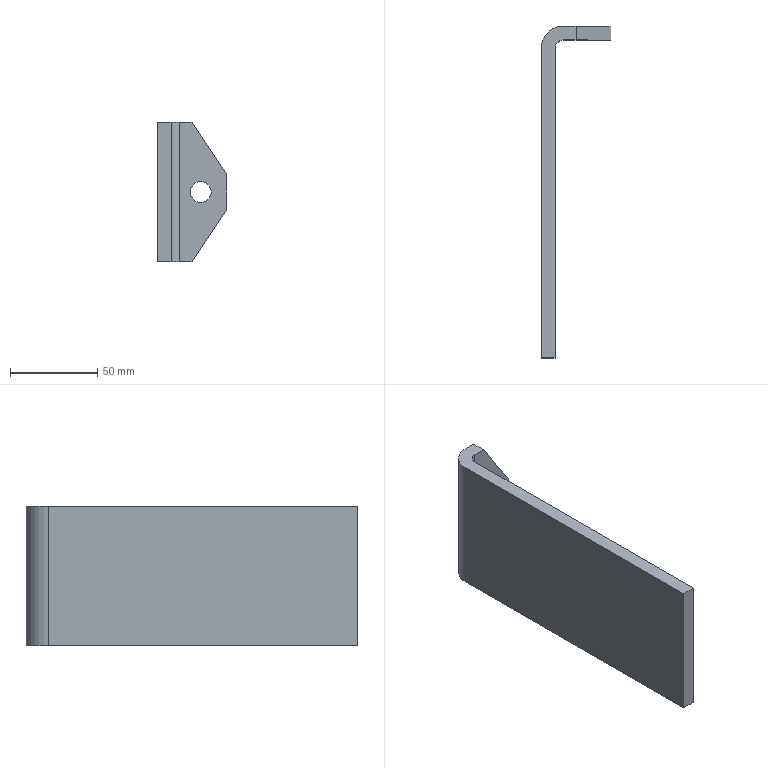Part | SolidWorks | features Extrusion 1, ICE 1 | 1 solid | 14 faces | box 40 x 190 x 80 mm | volume 133903 mm3 | plane 10 | cylinder 4 | commonest cylinder face diameters 12 x2 10 x1 26 x1
STEP:
#1=CARTESIAN_POINT('',(-15.,-8.,46.));
#2=VERTEX_POINT('',#1);
#3=CARTESIAN_POINT('',(-15.,-8.,34.));
#4=VERTEX_POINT('',#3);
#5=CARTESIAN_POINT('',(-15.,-8.,40.));
#6=DIRECTION('',(0.,-1.,0.));
#7=DIRECTION('',(0.,0.,-1.));
#8=AXIS2_PLACEMENT_3D('',#5,#6,#7);
#9=CIRCLE('',#8,6.);
#10=EDGE_CURVE('',#2,#4,#9,.T.);
#11=ORIENTED_EDGE('',*,*,#10,.T.);
#12=CARTESIAN_POINT('',(-15.,0.,34.));
#13=VERTEX_POINT('',#12);
#14=CARTESIAN_POINT('',(-15.,-12.,34.));
#15=DIRECTION('',(0.,1.,0.));
#16=VECTOR('',#15,1000.);
#17=LINE('',#14,#16);
#18=EDGE_CURVE('',#4,#13,#17,.T.);
#19=ORIENTED_EDGE('',*,*,#18,.T.);
#20=CARTESIAN_POINT('',(-15.,0.,46.));
#21=VERTEX_POINT('',#20);
#22=CARTESIAN_POINT('',(-15.,0.,40.));
#23=DIRECTION('',(0.,1.,0.));
#24=DIRECTION('',(0.,0.,1.));
#25=AXIS2_PLACEMENT_3D('',#22,#23,#24);
#26=CIRCLE('',#25,6.);
#27=EDGE_CURVE('',#13,#21,#26,.T.);
#28=ORIENTED_EDGE('',*,*,#27,.T.);
#29=CARTESIAN_POINT('',(-15.,-12.,46.));
#30=DIRECTION('',(0.,1.,0.));
#31=VECTOR('',#30,1000.);
#32=LINE('',#29,#31);
#33=EDGE_CURVE('',#2,#21,#32,.T.);
#34=ORIENTED_EDGE('',*,*,#33,.F.);
#35=EDGE_LOOP('',(#11,#19,#28,#34));
#36=FACE_OUTER_BOUND('',#35,.T.);
#37=CARTESIAN_POINT('',(-15.,-12.,40.));
#38=DIRECTION('',(0.,1.,0.));
#39=DIRECTION('',(0.,0.,1.));
#40=AXIS2_PLACEMENT_3D('',#37,#38,#39);
#41=CYLINDRICAL_SURFACE('',#40,6.);
#42=ADVANCED_FACE('',(#36),#41,.F.);
#43=ORIENTED_EDGE('',*,*,#10,.F.);
#44=CARTESIAN_POINT('',(-15.,-8.,40.));
#45=DIRECTION('',(0.,-1.,0.));
#46=DIRECTION('',(0.,0.,-1.));
#47=AXIS2_PLACEMENT_3D('',#44,#45,#46);
#48=CIRCLE('',#47,6.);
#49=EDGE_CURVE('',#4,#2,#48,.T.);
#50=ORIENTED_EDGE('',*,*,#49,.F.);
#51=EDGE_LOOP('',(#43,#50));
#52=FACE_BOUND('',#51,.T.);
#53=CARTESIAN_POINT('',(0.,-8.,50.));
#54=VERTEX_POINT('',#53);
#55=CARTESIAN_POINT('',(0.,-8.,30.));
#56=VERTEX_POINT('',#55);
#57=CARTESIAN_POINT('',(0.,-8.,80.));
#58=DIRECTION('',(0.,0.,-1.));
#59=VECTOR('',#58,1000.);
#60=LINE('',#57,#59);
#61=EDGE_CURVE('',#54,#56,#60,.T.);
#62=ORIENTED_EDGE('',*,*,#61,.F.);
#63=CARTESIAN_POINT('',(-20.,-8.,80.));
#64=VERTEX_POINT('',#63);
#65=CARTESIAN_POINT('',(-13.846,-8.,70.769));
#66=DIRECTION('',(-0.5547,0.,0.8321));
#67=VECTOR('',#66,1000.);
#68=LINE('',#65,#67);
#69=EDGE_CURVE('',#54,#64,#68,.T.);
#70=ORIENTED_EDGE('',*,*,#69,.T.);
#71=CARTESIAN_POINT('',(-27.,-8.,80.));
#72=VERTEX_POINT('',#71);
#73=CARTESIAN_POINT('',(0.,-8.,80.));
#74=DIRECTION('',(-1.,0.,0.));
#75=VECTOR('',#74,1000.);
#76=LINE('',#73,#75);
#77=EDGE_CURVE('',#64,#72,#76,.T.);
#78=ORIENTED_EDGE('',*,*,#77,.T.);
#79=CARTESIAN_POINT('',(-27.,-8.,0.));
#80=VERTEX_POINT('',#79);
#81=CARTESIAN_POINT('',(-27.,-8.,80.));
#82=DIRECTION('',(0.,0.,-1.));
#83=VECTOR('',#82,1000.);
#84=LINE('',#81,#83);
#85=EDGE_CURVE('',#72,#80,#84,.T.);
#86=ORIENTED_EDGE('',*,*,#85,.T.);
#87=CARTESIAN_POINT('',(-20.,-8.,0.));
#88=VERTEX_POINT('',#87);
#89=CARTESIAN_POINT('',(0.,-8.,0.));
#90=DIRECTION('',(-1.,0.,0.));
#91=VECTOR('',#90,1000.);
#92=LINE('',#89,#91);
#93=EDGE_CURVE('',#88,#80,#92,.T.);
#94=ORIENTED_EDGE('',*,*,#93,.F.);
#95=CARTESIAN_POINT('',(23.077,-8.,64.615));
#96=DIRECTION('',(-0.5547,0.,-0.8321));
#97=VECTOR('',#96,1000.);
#98=LINE('',#95,#97);
#99=EDGE_CURVE('',#56,#88,#98,.T.);
#100=ORIENTED_EDGE('',*,*,#99,.F.);
#101=EDGE_LOOP('',(#62,#70,#78,#86,#94,#100));
#102=FACE_OUTER_BOUND('',#101,.T.);
#103=CARTESIAN_POINT('',(0.,-8.,80.));
#104=DIRECTION('',(0.,-1.,0.));
#105=DIRECTION('',(0.,0.,-1.));
#106=AXIS2_PLACEMENT_3D('',#103,#104,#105);
#107=PLANE('',#106);
#108=ADVANCED_FACE('',(#52,#102),#107,.T.);
#109=CARTESIAN_POINT('',(0.,0.,50.));
#110=VERTEX_POINT('',#109);
#111=CARTESIAN_POINT('',(0.,0.,30.));
#112=VERTEX_POINT('',#111);
#113=CARTESIAN_POINT('',(0.,0.,80.));
#114=DIRECTION('',(0.,0.,-1.));
#115=VECTOR('',#114,1000.);
#116=LINE('',#113,#115);
#117=EDGE_CURVE('',#110,#112,#116,.T.);
#118=ORIENTED_EDGE('',*,*,#117,.F.);
#119=CARTESIAN_POINT('',(0.,-12.,50.));
#120=DIRECTION('',(0.,1.,0.));
#121=VECTOR('',#120,1000.);
#122=LINE('',#119,#121);
#123=EDGE_CURVE('',#54,#110,#122,.T.);
#124=ORIENTED_EDGE('',*,*,#123,.F.);
#125=ORIENTED_EDGE('',*,*,#61,.T.);
#126=CARTESIAN_POINT('',(0.,-12.,30.));
#127=DIRECTION('',(0.,1.,0.));
#128=VECTOR('',#127,1000.);
#129=LINE('',#126,#128);
#130=EDGE_CURVE('',#56,#112,#129,.T.);
#131=ORIENTED_EDGE('',*,*,#130,.T.);
#132=EDGE_LOOP('',(#118,#124,#125,#131));
#133=FACE_OUTER_BOUND('',#132,.T.);
#134=CARTESIAN_POINT('',(0.,0.,80.));
#135=DIRECTION('',(1.,0.,0.));
#136=DIRECTION('',(0.,0.,-1.));
#137=AXIS2_PLACEMENT_3D('',#134,#135,#136);
#138=PLANE('',#137);
#139=ADVANCED_FACE('',(#133),#138,.T.);
#140=CARTESIAN_POINT('',(-15.,0.,40.));
#141=DIRECTION('',(0.,1.,0.));
#142=DIRECTION('',(0.,0.,1.));
#143=AXIS2_PLACEMENT_3D('',#140,#141,#142);
#144=CIRCLE('',#143,6.);
#145=EDGE_CURVE('',#21,#13,#144,.T.);
#146=ORIENTED_EDGE('',*,*,#145,.F.);
#147=ORIENTED_EDGE('',*,*,#27,.F.);
#148=EDGE_LOOP('',(#146,#147));
#149=FACE_BOUND('',#148,.T.);
#150=CARTESIAN_POINT('',(-20.,0.,80.));
#151=VERTEX_POINT('',#150);
#152=CARTESIAN_POINT('',(-20.,0.,80.));
#153=DIRECTION('',(0.5547,0.,-0.8321));
#154=VECTOR('',#153,1000.);
#155=LINE('',#152,#154);
#156=EDGE_CURVE('',#151,#110,#155,.T.);
#157=ORIENTED_EDGE('',*,*,#156,.T.);
#158=ORIENTED_EDGE('',*,*,#117,.T.);
#159=CARTESIAN_POINT('',(-20.,0.,0.));
#160=VERTEX_POINT('',#159);
#161=CARTESIAN_POINT('',(-20.,0.,0.));
#162=DIRECTION('',(0.5547,0.,0.8321));
#163=VECTOR('',#162,1000.);
#164=LINE('',#161,#163);
#165=EDGE_CURVE('',#160,#112,#164,.T.);
#166=ORIENTED_EDGE('',*,*,#165,.F.);
#167=CARTESIAN_POINT('',(-27.,0.,0.));
#168=VERTEX_POINT('',#167);
#169=CARTESIAN_POINT('',(0.,0.,0.));
#170=DIRECTION('',(-1.,0.,0.));
#171=VECTOR('',#170,1000.);
#172=LINE('',#169,#171);
#173=EDGE_CURVE('',#160,#168,#172,.T.);
#174=ORIENTED_EDGE('',*,*,#173,.T.);
#175=CARTESIAN_POINT('',(-27.,0.,80.));
#176=VERTEX_POINT('',#175);
#177=CARTESIAN_POINT('',(-27.,0.,80.));
#178=DIRECTION('',(0.,0.,-1.));
#179=VECTOR('',#178,1000.);
#180=LINE('',#177,#179);
#181=EDGE_CURVE('',#176,#168,#180,.T.);
#182=ORIENTED_EDGE('',*,*,#181,.F.);
#183=CARTESIAN_POINT('',(0.,0.,80.));
#184=DIRECTION('',(-1.,0.,0.));
#185=VECTOR('',#184,1000.);
#186=LINE('',#183,#185);
#187=EDGE_CURVE('',#151,#176,#186,.T.);
#188=ORIENTED_EDGE('',*,*,#187,.F.);
#189=EDGE_LOOP('',(#157,#158,#166,#174,#182,#188));
#190=FACE_OUTER_BOUND('',#189,.T.);
#191=CARTESIAN_POINT('',(0.,0.,80.));
#192=DIRECTION('',(0.,-1.,0.));
#193=DIRECTION('',(0.,0.,-1.));
#194=AXIS2_PLACEMENT_3D('',#191,#192,#193);
#195=PLANE('',#194);
#196=ADVANCED_FACE('',(#149,#190),#195,.F.);
#197=ORIENTED_EDGE('',*,*,#77,.F.);
#198=CARTESIAN_POINT('',(-20.,-13.,80.));
#199=DIRECTION('',(0.,1.,0.));
#200=VECTOR('',#199,1000.);
#201=LINE('',#198,#200);
#202=EDGE_CURVE('',#64,#151,#201,.T.);
#203=ORIENTED_EDGE('',*,*,#202,.T.);
#204=ORIENTED_EDGE('',*,*,#187,.T.);
#205=CARTESIAN_POINT('',(-40.,-13.,80.));
#206=VERTEX_POINT('',#205);
#207=CARTESIAN_POINT('',(-27.,-13.,80.));
#208=DIRECTION('',(0.,0.,1.));
#209=DIRECTION('',(1.,0.,0.));
#210=AXIS2_PLACEMENT_3D('',#207,#208,#209);
#211=CIRCLE('',#210,13.);
#212=EDGE_CURVE('',#176,#206,#211,.T.);
#213=ORIENTED_EDGE('',*,*,#212,.T.);
#214=CARTESIAN_POINT('',(-40.,-190.,80.));
#215=VERTEX_POINT('',#214);
#216=CARTESIAN_POINT('',(-40.,-13.,80.));
#217=DIRECTION('',(0.,-1.,0.));
#218=VECTOR('',#217,1000.);
#219=LINE('',#216,#218);
#220=EDGE_CURVE('',#206,#215,#219,.T.);
#221=ORIENTED_EDGE('',*,*,#220,.T.);
#222=CARTESIAN_POINT('',(-32.,-190.,80.));
#223=VERTEX_POINT('',#222);
#224=CARTESIAN_POINT('',(-40.,-190.,80.));
#225=DIRECTION('',(1.,0.,0.));
#226=VECTOR('',#225,1000.);
#227=LINE('',#224,#226);
#228=EDGE_CURVE('',#215,#223,#227,.T.);
#229=ORIENTED_EDGE('',*,*,#228,.T.);
#230=CARTESIAN_POINT('',(-32.,-13.,80.));
#231=VERTEX_POINT('',#230);
#232=CARTESIAN_POINT('',(-32.,-13.,80.));
#233=DIRECTION('',(0.,-1.,0.));
#234=VECTOR('',#233,1000.);
#235=LINE('',#232,#234);
#236=EDGE_CURVE('',#231,#223,#235,.T.);
#237=ORIENTED_EDGE('',*,*,#236,.F.);
#238=CARTESIAN_POINT('',(-27.,-13.,80.));
#239=DIRECTION('',(0.,0.,1.));
#240=DIRECTION('',(1.,0.,0.));
#241=AXIS2_PLACEMENT_3D('',#238,#239,#240);
#242=CIRCLE('',#241,5.);
#243=EDGE_CURVE('',#72,#231,#242,.T.);
#244=ORIENTED_EDGE('',*,*,#243,.F.);
#245=EDGE_LOOP('',(#197,#203,#204,#213,#221,#229,#237,#244));
#246=FACE_OUTER_BOUND('',#245,.T.);
#247=CARTESIAN_POINT('',(-27.,-13.,80.));
#248=DIRECTION('',(0.,0.,1.));
#249=DIRECTION('',(1.,0.,0.));
#250=AXIS2_PLACEMENT_3D('',#247,#248,#249);
#251=PLANE('',#250);
#252=ADVANCED_FACE('',(#246),#251,.T.);
#253=CARTESIAN_POINT('',(-40.,-13.,0.));
#254=VERTEX_POINT('',#253);
#255=CARTESIAN_POINT('',(-40.,-190.,0.));
#256=VERTEX_POINT('',#255);
#257=CARTESIAN_POINT('',(-40.,-13.,0.));
#258=DIRECTION('',(0.,-1.,0.));
#259=VECTOR('',#258,1000.);
#260=LINE('',#257,#259);
#261=EDGE_CURVE('',#254,#256,#260,.T.);
#262=ORIENTED_EDGE('',*,*,#261,.T.);
#263=CARTESIAN_POINT('',(-40.,-190.,80.));
#264=DIRECTION('',(0.,0.,-1.));
#265=VECTOR('',#264,1000.);
#266=LINE('',#263,#265);
#267=EDGE_CURVE('',#215,#256,#266,.T.);
#268=ORIENTED_EDGE('',*,*,#267,.F.);
#269=ORIENTED_EDGE('',*,*,#220,.F.);
#270=CARTESIAN_POINT('',(-40.,-13.,80.));
#271=DIRECTION('',(0.,0.,-1.));
#272=VECTOR('',#271,1000.);
#273=LINE('',#270,#272);
#274=EDGE_CURVE('',#206,#254,#273,.T.);
#275=ORIENTED_EDGE('',*,*,#274,.T.);
#276=EDGE_LOOP('',(#262,#268,#269,#275));
#277=FACE_OUTER_BOUND('',#276,.T.);
#278=CARTESIAN_POINT('',(-40.,-13.,80.));
#279=DIRECTION('',(1.,0.,0.));
#280=DIRECTION('',(0.,1.,0.));
#281=AXIS2_PLACEMENT_3D('',#278,#279,#280);
#282=PLANE('',#281);
#283=ADVANCED_FACE('',(#277),#282,.F.);
#284=CARTESIAN_POINT('',(-32.,-190.,0.));
#285=VERTEX_POINT('',#284);
#286=CARTESIAN_POINT('',(-40.,-190.,0.));
#287=DIRECTION('',(1.,0.,0.));
#288=VECTOR('',#287,1000.);
#289=LINE('',#286,#288);
#290=EDGE_CURVE('',#256,#285,#289,.T.);
#291=ORIENTED_EDGE('',*,*,#290,.T.);
#292=CARTESIAN_POINT('',(-32.,-190.,80.));
#293=DIRECTION('',(0.,0.,-1.));
#294=VECTOR('',#293,1000.);
#295=LINE('',#292,#294);
#296=EDGE_CURVE('',#223,#285,#295,.T.);
#297=ORIENTED_EDGE('',*,*,#296,.F.);
#298=ORIENTED_EDGE('',*,*,#228,.F.);
#299=ORIENTED_EDGE('',*,*,#267,.T.);
#300=EDGE_LOOP('',(#291,#297,#298,#299));
#301=FACE_OUTER_BOUND('',#300,.T.);
#302=CARTESIAN_POINT('',(-40.,-190.,80.));
#303=DIRECTION('',(0.,1.,0.));
#304=DIRECTION('',(0.,0.,1.));
#305=AXIS2_PLACEMENT_3D('',#302,#303,#304);
#306=PLANE('',#305);
#307=ADVANCED_FACE('',(#301),#306,.F.);
#308=CARTESIAN_POINT('',(-32.,-13.,0.));
#309=VERTEX_POINT('',#308);
#310=CARTESIAN_POINT('',(-32.,-13.,0.));
#311=DIRECTION('',(0.,-1.,0.));
#312=VECTOR('',#311,1000.);
#313=LINE('',#310,#312);
#314=EDGE_CURVE('',#309,#285,#313,.T.);
#315=ORIENTED_EDGE('',*,*,#314,.F.);
#316=CARTESIAN_POINT('',(-32.,-13.,80.));
#317=DIRECTION('',(0.,0.,-1.));
#318=VECTOR('',#317,1000.);
#319=LINE('',#316,#318);
#320=EDGE_CURVE('',#231,#309,#319,.T.);
#321=ORIENTED_EDGE('',*,*,#320,.F.);
#322=ORIENTED_EDGE('',*,*,#236,.T.);
#323=ORIENTED_EDGE('',*,*,#296,.T.);
#324=EDGE_LOOP('',(#315,#321,#322,#323));
#325=FACE_OUTER_BOUND('',#324,.T.);
#326=CARTESIAN_POINT('',(-32.,-13.,80.));
#327=DIRECTION('',(1.,0.,0.));
#328=DIRECTION('',(0.,0.,-1.));
#329=AXIS2_PLACEMENT_3D('',#326,#327,#328);
#330=PLANE('',#329);
#331=ADVANCED_FACE('',(#325),#330,.T.);
#332=CARTESIAN_POINT('',(-27.,-13.,0.));
#333=DIRECTION('',(0.,0.,1.));
#334=DIRECTION('',(1.,0.,0.));
#335=AXIS2_PLACEMENT_3D('',#332,#333,#334);
#336=CIRCLE('',#335,5.);
#337=EDGE_CURVE('',#80,#309,#336,.T.);
#338=ORIENTED_EDGE('',*,*,#337,.F.);
#339=ORIENTED_EDGE('',*,*,#85,.F.);
#340=ORIENTED_EDGE('',*,*,#243,.T.);
#341=ORIENTED_EDGE('',*,*,#320,.T.);
#342=EDGE_LOOP('',(#338,#339,#340,#341));
#343=FACE_OUTER_BOUND('',#342,.T.);
#344=CARTESIAN_POINT('',(-27.,-13.,80.));
#345=DIRECTION('',(0.,0.,-1.));
#346=DIRECTION('',(-1.,0.,0.));
#347=AXIS2_PLACEMENT_3D('',#344,#345,#346);
#348=CYLINDRICAL_SURFACE('',#347,5.);
#349=ADVANCED_FACE('',(#343),#348,.F.);
#350=CARTESIAN_POINT('',(-27.,-13.,0.));
#351=DIRECTION('',(0.,0.,1.));
#352=DIRECTION('',(1.,0.,0.));
#353=AXIS2_PLACEMENT_3D('',#350,#351,#352);
#354=CIRCLE('',#353,13.);
#355=EDGE_CURVE('',#168,#254,#354,.T.);
#356=ORIENTED_EDGE('',*,*,#355,.T.);
#357=ORIENTED_EDGE('',*,*,#274,.F.);
#358=ORIENTED_EDGE('',*,*,#212,.F.);
#359=ORIENTED_EDGE('',*,*,#181,.T.);
#360=EDGE_LOOP('',(#356,#357,#358,#359));
#361=FACE_OUTER_BOUND('',#360,.T.);
#362=CARTESIAN_POINT('',(-27.,-13.,80.));
#363=DIRECTION('',(0.,0.,-1.));
#364=DIRECTION('',(-1.,0.,0.));
#365=AXIS2_PLACEMENT_3D('',#362,#363,#364);
#366=CYLINDRICAL_SURFACE('',#365,13.);
#367=ADVANCED_FACE('',(#361),#366,.T.);
#368=ORIENTED_EDGE('',*,*,#173,.F.);
#369=CARTESIAN_POINT('',(-20.,-13.,0.));
#370=DIRECTION('',(0.,-1.,0.));
#371=VECTOR('',#370,1000.);
#372=LINE('',#369,#371);
#373=EDGE_CURVE('',#160,#88,#372,.T.);
#374=ORIENTED_EDGE('',*,*,#373,.T.);
#375=ORIENTED_EDGE('',*,*,#93,.T.);
#376=ORIENTED_EDGE('',*,*,#337,.T.);
#377=ORIENTED_EDGE('',*,*,#314,.T.);
#378=ORIENTED_EDGE('',*,*,#290,.F.);
#379=ORIENTED_EDGE('',*,*,#261,.F.);
#380=ORIENTED_EDGE('',*,*,#355,.F.);
#381=EDGE_LOOP('',(#368,#374,#375,#376,#377,#378,#379,#380));
#382=FACE_OUTER_BOUND('',#381,.T.);
#383=CARTESIAN_POINT('',(-27.,-13.,0.));
#384=DIRECTION('',(0.,0.,1.));
#385=DIRECTION('',(1.,0.,0.));
#386=AXIS2_PLACEMENT_3D('',#383,#384,#385);
#387=PLANE('',#386);
#388=ADVANCED_FACE('',(#382),#387,.F.);
#389=ORIENTED_EDGE('',*,*,#99,.T.);
#390=ORIENTED_EDGE('',*,*,#373,.F.);
#391=ORIENTED_EDGE('',*,*,#165,.T.);
#392=ORIENTED_EDGE('',*,*,#130,.F.);
#393=EDGE_LOOP('',(#389,#390,#391,#392));
#394=FACE_OUTER_BOUND('',#393,.T.);
#395=CARTESIAN_POINT('',(-20.,-12.,0.));
#396=DIRECTION('',(-0.8321,0.,0.5547));
#397=DIRECTION('',(0.5547,0.,0.8321));
#398=AXIS2_PLACEMENT_3D('',#395,#396,#397);
#399=PLANE('',#398);
#400=ADVANCED_FACE('',(#394),#399,.F.);
#401=ORIENTED_EDGE('',*,*,#123,.T.);
#402=ORIENTED_EDGE('',*,*,#156,.F.);
#403=ORIENTED_EDGE('',*,*,#202,.F.);
#404=ORIENTED_EDGE('',*,*,#69,.F.);
#405=EDGE_LOOP('',(#401,#402,#403,#404));
#406=FACE_OUTER_BOUND('',#405,.T.);
#407=CARTESIAN_POINT('',(-20.,-12.,80.));
#408=DIRECTION('',(0.8321,0.,0.5547));
#409=DIRECTION('',(0.5547,0.,-0.8321));
#410=AXIS2_PLACEMENT_3D('',#407,#408,#409);
#411=PLANE('',#410);
#412=ADVANCED_FACE('',(#406),#411,.T.);
#413=ORIENTED_EDGE('',*,*,#18,.F.);
#414=ORIENTED_EDGE('',*,*,#49,.T.);
#415=ORIENTED_EDGE('',*,*,#33,.T.);
#416=ORIENTED_EDGE('',*,*,#145,.T.);
#417=EDGE_LOOP('',(#413,#414,#415,#416));
#418=FACE_OUTER_BOUND('',#417,.T.);
#419=CARTESIAN_POINT('',(-15.,-12.,40.));
#420=DIRECTION('',(0.,1.,0.));
#421=DIRECTION('',(0.,0.,1.));
#422=AXIS2_PLACEMENT_3D('',#419,#420,#421);
#423=CYLINDRICAL_SURFACE('',#422,6.);
#424=ADVANCED_FACE('',(#418),#423,.F.);
#425=CLOSED_SHELL('',(#42,#108,#139,#196,#252,#283,#307,#331,#349,#367,#388,#400,#412,#424));
#426=MANIFOLD_SOLID_BREP('',#425);
#427=CARTESIAN_POINT('',(0.,0.,0.));
#428=DIRECTION('',(0.,0.,1.));
#429=DIRECTION('',(1.,0.,0.));
#430=AXIS2_PLACEMENT_3D('',#427,#428,#429);
#431=(LENGTH_UNIT()NAMED_UNIT(*)SI_UNIT(.MILLI.,.METRE.));
#432=UNCERTAINTY_MEASURE_WITH_UNIT(LENGTH_MEASURE(0.00001),#431,'','');
#433=(NAMED_UNIT(*)PLANE_ANGLE_UNIT()SI_UNIT($,.RADIAN.));
#434=(NAMED_UNIT(*)SI_UNIT($,.STERADIAN.)SOLID_ANGLE_UNIT());
#435=(GEOMETRIC_REPRESENTATION_CONTEXT(3)GLOBAL_UNCERTAINTY_ASSIGNED_CONTEXT((#432))GLOBAL_UNIT_ASSIGNED_CONTEXT((#431,#433,#434))REPRESENTATION_CONTEXT('',''));
#436=ADVANCED_BREP_SHAPE_REPRESENTATION('',(#426,#430),#435);